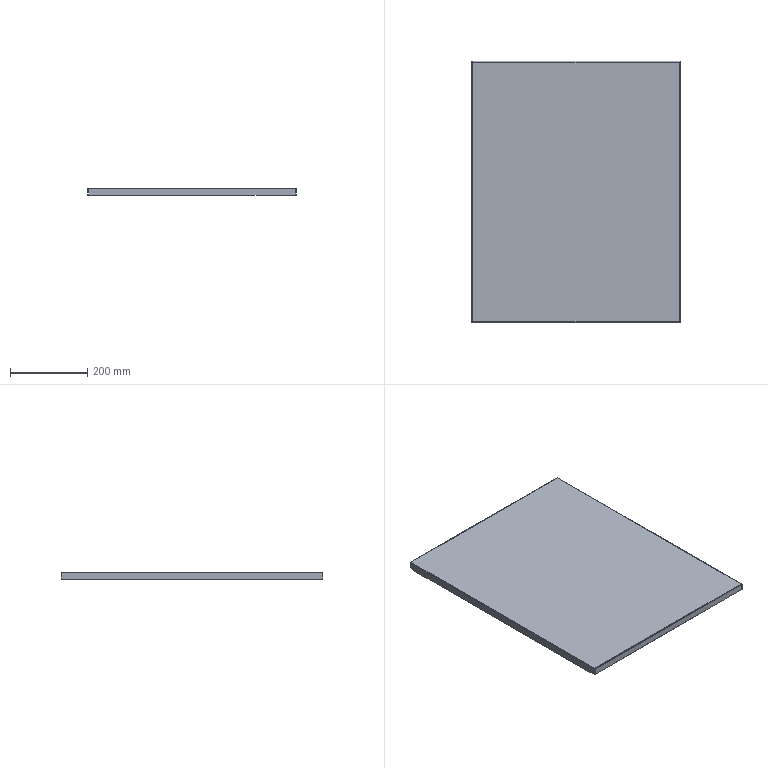Part | SolidWorks | features BaseBody 1 | 1 solid | 50 faces | box 537.5 x 674.5 x 20 mm | volume 485472 mm3 | plane 42 | cylinder 8 | commonest cylinder face diameters 1 x4 3.4 x4
STEP:
#1=CARTESIAN_POINT('',(-267.55,-319.25,-20.));
#2=VERTEX_POINT('',#1);
#3=CARTESIAN_POINT('',(-268.75,-319.25,-20.));
#4=VERTEX_POINT('',#3);
#5=CARTESIAN_POINT('',(268.75,-319.25,-20.));
#6=DIRECTION('',(-1.,0.,0.));
#7=VECTOR('',#6,1000.);
#8=LINE('',#5,#7);
#9=EDGE_CURVE('',#2,#4,#8,.T.);
#10=ORIENTED_EDGE('',*,*,#9,.F.);
#11=CARTESIAN_POINT('',(-267.55,-319.25,-18.));
#12=VERTEX_POINT('',#11);
#13=CARTESIAN_POINT('',(-267.55,-319.25,0.));
#14=DIRECTION('',(0.,0.,1.));
#15=VECTOR('',#14,1000.);
#16=LINE('',#13,#15);
#17=EDGE_CURVE('',#2,#12,#16,.T.);
#18=ORIENTED_EDGE('',*,*,#17,.T.);
#19=CARTESIAN_POINT('',(-268.75,-319.25,-18.));
#20=VERTEX_POINT('',#19);
#21=CARTESIAN_POINT('',(268.75,-319.25,-18.));
#22=DIRECTION('',(-1.,0.,0.));
#23=VECTOR('',#22,1000.);
#24=LINE('',#21,#23);
#25=EDGE_CURVE('',#12,#20,#24,.T.);
#26=ORIENTED_EDGE('',*,*,#25,.T.);
#27=CARTESIAN_POINT('',(-268.75,-319.25,0.));
#28=DIRECTION('',(0.,0.,1.));
#29=VECTOR('',#28,1000.);
#30=LINE('',#27,#29);
#31=EDGE_CURVE('',#4,#20,#30,.T.);
#32=ORIENTED_EDGE('',*,*,#31,.F.);
#33=EDGE_LOOP('',(#10,#18,#26,#32));
#34=FACE_OUTER_BOUND('',#33,.T.);
#35=CARTESIAN_POINT('',(268.75,-319.25,-20.));
#36=DIRECTION('',(0.,1.,0.));
#37=DIRECTION('',(1.,0.,0.));
#38=AXIS2_PLACEMENT_3D('',#35,#36,#37);
#39=PLANE('',#38);
#40=ADVANCED_FACE('',(#34),#39,.F.);
#41=ORIENTED_EDGE('',*,*,#25,.F.);
#42=CARTESIAN_POINT('',(-267.55,-337.25,-18.));
#43=VERTEX_POINT('',#42);
#44=CARTESIAN_POINT('',(-267.55,0.,-18.));
#45=DIRECTION('',(0.,-1.,0.));
#46=VECTOR('',#45,1000.);
#47=LINE('',#44,#46);
#48=EDGE_CURVE('',#12,#43,#47,.T.);
#49=ORIENTED_EDGE('',*,*,#48,.T.);
#50=CARTESIAN_POINT('',(-268.75,-337.25,-18.));
#51=VERTEX_POINT('',#50);
#52=CARTESIAN_POINT('',(268.75,-337.25,-18.));
#53=DIRECTION('',(-1.,0.,0.));
#54=VECTOR('',#53,1000.);
#55=LINE('',#52,#54);
#56=EDGE_CURVE('',#43,#51,#55,.T.);
#57=ORIENTED_EDGE('',*,*,#56,.T.);
#58=CARTESIAN_POINT('',(-268.75,0.,-18.));
#59=DIRECTION('',(0.,-1.,0.));
#60=VECTOR('',#59,1000.);
#61=LINE('',#58,#60);
#62=EDGE_CURVE('',#20,#51,#61,.T.);
#63=ORIENTED_EDGE('',*,*,#62,.F.);
#64=EDGE_LOOP('',(#41,#49,#57,#63));
#65=FACE_OUTER_BOUND('',#64,.T.);
#66=CARTESIAN_POINT('',(268.75,-337.25,-18.));
#67=DIRECTION('',(0.,0.,1.));
#68=DIRECTION('',(1.,0.,0.));
#69=AXIS2_PLACEMENT_3D('',#66,#67,#68);
#70=PLANE('',#69);
#71=ADVANCED_FACE('',(#65),#70,.F.);
#72=CARTESIAN_POINT('',(-267.55,319.25,-18.));
#73=VERTEX_POINT('',#72);
#74=CARTESIAN_POINT('',(-268.75,319.25,-18.));
#75=VERTEX_POINT('',#74);
#76=CARTESIAN_POINT('',(268.75,319.25,-18.));
#77=DIRECTION('',(-1.,0.,0.));
#78=VECTOR('',#77,1000.);
#79=LINE('',#76,#78);
#80=EDGE_CURVE('',#73,#75,#79,.T.);
#81=ORIENTED_EDGE('',*,*,#80,.F.);
#82=CARTESIAN_POINT('',(-267.55,319.25,-20.));
#83=VERTEX_POINT('',#82);
#84=CARTESIAN_POINT('',(-267.55,319.25,0.));
#85=DIRECTION('',(0.,0.,-1.));
#86=VECTOR('',#85,1000.);
#87=LINE('',#84,#86);
#88=EDGE_CURVE('',#73,#83,#87,.T.);
#89=ORIENTED_EDGE('',*,*,#88,.T.);
#90=CARTESIAN_POINT('',(-268.75,319.25,-20.));
#91=VERTEX_POINT('',#90);
#92=CARTESIAN_POINT('',(268.75,319.25,-20.));
#93=DIRECTION('',(-1.,0.,0.));
#94=VECTOR('',#93,1000.);
#95=LINE('',#92,#94);
#96=EDGE_CURVE('',#83,#91,#95,.T.);
#97=ORIENTED_EDGE('',*,*,#96,.T.);
#98=CARTESIAN_POINT('',(-268.75,319.25,0.));
#99=DIRECTION('',(0.,0.,-1.));
#100=VECTOR('',#99,1000.);
#101=LINE('',#98,#100);
#102=EDGE_CURVE('',#75,#91,#101,.T.);
#103=ORIENTED_EDGE('',*,*,#102,.F.);
#104=EDGE_LOOP('',(#81,#89,#97,#103));
#105=FACE_OUTER_BOUND('',#104,.T.);
#106=CARTESIAN_POINT('',(268.75,319.25,-20.));
#107=DIRECTION('',(0.,-1.,0.));
#108=DIRECTION('',(0.,0.,-1.));
#109=AXIS2_PLACEMENT_3D('',#106,#107,#108);
#110=PLANE('',#109);
#111=ADVANCED_FACE('',(#105),#110,.F.);
#112=CARTESIAN_POINT('',(-267.55,337.25,-18.));
#113=VERTEX_POINT('',#112);
#114=CARTESIAN_POINT('',(-268.75,337.25,-18.));
#115=VERTEX_POINT('',#114);
#116=CARTESIAN_POINT('',(268.75,337.25,-18.));
#117=DIRECTION('',(-1.,0.,0.));
#118=VECTOR('',#117,1000.);
#119=LINE('',#116,#118);
#120=EDGE_CURVE('',#113,#115,#119,.T.);
#121=ORIENTED_EDGE('',*,*,#120,.F.);
#122=CARTESIAN_POINT('',(-267.55,0.,-18.));
#123=DIRECTION('',(0.,-1.,0.));
#124=VECTOR('',#123,1000.);
#125=LINE('',#122,#124);
#126=EDGE_CURVE('',#113,#73,#125,.T.);
#127=ORIENTED_EDGE('',*,*,#126,.T.);
#128=ORIENTED_EDGE('',*,*,#80,.T.);
#129=CARTESIAN_POINT('',(-268.75,0.,-18.));
#130=DIRECTION('',(0.,-1.,0.));
#131=VECTOR('',#130,1000.);
#132=LINE('',#129,#131);
#133=EDGE_CURVE('',#115,#75,#132,.T.);
#134=ORIENTED_EDGE('',*,*,#133,.F.);
#135=EDGE_LOOP('',(#121,#127,#128,#134));
#136=FACE_OUTER_BOUND('',#135,.T.);
#137=CARTESIAN_POINT('',(268.75,337.25,-18.));
#138=DIRECTION('',(0.,0.,1.));
#139=DIRECTION('',(1.,0.,0.));
#140=AXIS2_PLACEMENT_3D('',#137,#138,#139);
#141=PLANE('',#140);
#142=ADVANCED_FACE('',(#136),#141,.F.);
#143=CARTESIAN_POINT('',(267.55,-335.55,-18.));
#144=VERTEX_POINT('',#143);
#145=CARTESIAN_POINT('',(267.55,-319.25,-18.));
#146=VERTEX_POINT('',#145);
#147=CARTESIAN_POINT('',(267.55,0.,-18.));
#148=DIRECTION('',(0.,1.,0.));
#149=VECTOR('',#148,1000.);
#150=LINE('',#147,#149);
#151=EDGE_CURVE('',#144,#146,#150,.T.);
#152=ORIENTED_EDGE('',*,*,#151,.T.);
#153=CARTESIAN_POINT('',(268.75,-319.25,-18.));
#154=VERTEX_POINT('',#153);
#155=CARTESIAN_POINT('',(268.75,-319.25,-18.));
#156=DIRECTION('',(-1.,0.,0.));
#157=VECTOR('',#156,1000.);
#158=LINE('',#155,#157);
#159=EDGE_CURVE('',#154,#146,#158,.T.);
#160=ORIENTED_EDGE('',*,*,#159,.F.);
#161=CARTESIAN_POINT('',(268.75,-335.55,-18.));
#162=VERTEX_POINT('',#161);
#163=CARTESIAN_POINT('',(268.75,-337.25,-18.));
#164=DIRECTION('',(0.,1.,0.));
#165=VECTOR('',#164,1000.);
#166=LINE('',#163,#165);
#167=EDGE_CURVE('',#162,#154,#166,.T.);
#168=ORIENTED_EDGE('',*,*,#167,.F.);
#169=CARTESIAN_POINT('',(268.75,-335.55,-18.));
#170=DIRECTION('',(1.,0.,0.));
#171=VECTOR('',#170,1000.);
#172=LINE('',#169,#171);
#173=EDGE_CURVE('',#144,#162,#172,.T.);
#174=ORIENTED_EDGE('',*,*,#173,.F.);
#175=EDGE_LOOP('',(#152,#160,#168,#174));
#176=FACE_OUTER_BOUND('',#175,.T.);
#177=CARTESIAN_POINT('',(268.75,-337.25,-18.));
#178=DIRECTION('',(0.,0.,1.));
#179=DIRECTION('',(1.,0.,0.));
#180=AXIS2_PLACEMENT_3D('',#177,#178,#179);
#181=PLANE('',#180);
#182=ADVANCED_FACE('',(#176),#181,.F.);
#183=CARTESIAN_POINT('',(267.55,-319.25,-20.));
#184=VERTEX_POINT('',#183);
#185=CARTESIAN_POINT('',(267.55,-319.25,0.));
#186=DIRECTION('',(0.,0.,-1.));
#187=VECTOR('',#186,1000.);
#188=LINE('',#185,#187);
#189=EDGE_CURVE('',#146,#184,#188,.T.);
#190=ORIENTED_EDGE('',*,*,#189,.T.);
#191=CARTESIAN_POINT('',(268.75,-319.25,-20.));
#192=VERTEX_POINT('',#191);
#193=CARTESIAN_POINT('',(268.75,-319.25,-20.));
#194=DIRECTION('',(-1.,0.,0.));
#195=VECTOR('',#194,1000.);
#196=LINE('',#193,#195);
#197=EDGE_CURVE('',#192,#184,#196,.T.);
#198=ORIENTED_EDGE('',*,*,#197,.F.);
#199=CARTESIAN_POINT('',(268.75,-319.25,-20.));
#200=DIRECTION('',(0.,0.,-1.));
#201=VECTOR('',#200,1000.);
#202=LINE('',#199,#201);
#203=EDGE_CURVE('',#154,#192,#202,.T.);
#204=ORIENTED_EDGE('',*,*,#203,.F.);
#205=ORIENTED_EDGE('',*,*,#159,.T.);
#206=EDGE_LOOP('',(#190,#198,#204,#205));
#207=FACE_OUTER_BOUND('',#206,.T.);
#208=CARTESIAN_POINT('',(268.75,-319.25,-20.));
#209=DIRECTION('',(0.,1.,0.));
#210=DIRECTION('',(1.,0.,0.));
#211=AXIS2_PLACEMENT_3D('',#208,#209,#210);
#212=PLANE('',#211);
#213=ADVANCED_FACE('',(#207),#212,.F.);
#214=CARTESIAN_POINT('',(268.75,319.25,-18.));
#215=VERTEX_POINT('',#214);
#216=CARTESIAN_POINT('',(268.75,335.55,-18.));
#217=VERTEX_POINT('',#216);
#218=CARTESIAN_POINT('',(268.75,337.25,-18.));
#219=DIRECTION('',(0.,1.,0.));
#220=VECTOR('',#219,1000.);
#221=LINE('',#218,#220);
#222=EDGE_CURVE('',#215,#217,#221,.T.);
#223=ORIENTED_EDGE('',*,*,#222,.F.);
#224=CARTESIAN_POINT('',(267.55,319.25,-18.));
#225=VERTEX_POINT('',#224);
#226=CARTESIAN_POINT('',(268.75,319.25,-18.));
#227=DIRECTION('',(-1.,0.,0.));
#228=VECTOR('',#227,1000.);
#229=LINE('',#226,#228);
#230=EDGE_CURVE('',#215,#225,#229,.T.);
#231=ORIENTED_EDGE('',*,*,#230,.T.);
#232=CARTESIAN_POINT('',(267.55,335.55,-18.));
#233=VERTEX_POINT('',#232);
#234=CARTESIAN_POINT('',(267.55,0.,-18.));
#235=DIRECTION('',(0.,1.,0.));
#236=VECTOR('',#235,1000.);
#237=LINE('',#234,#236);
#238=EDGE_CURVE('',#225,#233,#237,.T.);
#239=ORIENTED_EDGE('',*,*,#238,.T.);
#240=CARTESIAN_POINT('',(268.75,335.55,-18.));
#241=DIRECTION('',(-1.,0.,0.));
#242=VECTOR('',#241,1000.);
#243=LINE('',#240,#242);
#244=EDGE_CURVE('',#217,#233,#243,.T.);
#245=ORIENTED_EDGE('',*,*,#244,.F.);
#246=EDGE_LOOP('',(#223,#231,#239,#245));
#247=FACE_OUTER_BOUND('',#246,.T.);
#248=CARTESIAN_POINT('',(268.75,337.25,-18.));
#249=DIRECTION('',(0.,0.,1.));
#250=DIRECTION('',(1.,0.,0.));
#251=AXIS2_PLACEMENT_3D('',#248,#249,#250);
#252=PLANE('',#251);
#253=ADVANCED_FACE('',(#247),#252,.F.);
#254=CARTESIAN_POINT('',(267.55,319.25,-20.));
#255=VERTEX_POINT('',#254);
#256=CARTESIAN_POINT('',(267.55,319.25,0.));
#257=DIRECTION('',(0.,0.,1.));
#258=VECTOR('',#257,1000.);
#259=LINE('',#256,#258);
#260=EDGE_CURVE('',#255,#225,#259,.T.);
#261=ORIENTED_EDGE('',*,*,#260,.T.);
#262=ORIENTED_EDGE('',*,*,#230,.F.);
#263=CARTESIAN_POINT('',(268.75,319.25,-20.));
#264=VERTEX_POINT('',#263);
#265=CARTESIAN_POINT('',(268.75,319.25,-20.));
#266=DIRECTION('',(0.,0.,1.));
#267=VECTOR('',#266,1000.);
#268=LINE('',#265,#267);
#269=EDGE_CURVE('',#264,#215,#268,.T.);
#270=ORIENTED_EDGE('',*,*,#269,.F.);
#271=CARTESIAN_POINT('',(268.75,319.25,-20.));
#272=DIRECTION('',(-1.,0.,0.));
#273=VECTOR('',#272,1000.);
#274=LINE('',#271,#273);
#275=EDGE_CURVE('',#264,#255,#274,.T.);
#276=ORIENTED_EDGE('',*,*,#275,.T.);
#277=EDGE_LOOP('',(#261,#262,#270,#276));
#278=FACE_OUTER_BOUND('',#277,.T.);
#279=CARTESIAN_POINT('',(268.75,319.25,-20.));
#280=DIRECTION('',(0.,-1.,0.));
#281=DIRECTION('',(0.,0.,-1.));
#282=AXIS2_PLACEMENT_3D('',#279,#280,#281);
#283=PLANE('',#282);
#284=ADVANCED_FACE('',(#278),#283,.F.);
#285=CARTESIAN_POINT('',(268.75,0.,-20.));
#286=DIRECTION('',(0.,1.,0.));
#287=VECTOR('',#286,1000.);
#288=LINE('',#285,#287);
#289=EDGE_CURVE('',#192,#264,#288,.T.);
#290=ORIENTED_EDGE('',*,*,#289,.F.);
#291=ORIENTED_EDGE('',*,*,#197,.T.);
#292=CARTESIAN_POINT('',(267.55,335.55,-20.));
#293=DIRECTION('',(0.,1.,0.));
#294=VECTOR('',#293,1000.);
#295=LINE('',#292,#294);
#296=EDGE_CURVE('',#184,#255,#295,.T.);
#297=ORIENTED_EDGE('',*,*,#296,.T.);
#298=ORIENTED_EDGE('',*,*,#275,.F.);
#299=EDGE_LOOP('',(#290,#291,#297,#298));
#300=FACE_OUTER_BOUND('',#299,.T.);
#301=CARTESIAN_POINT('',(268.75,335.55,-20.));
#302=DIRECTION('',(0.,0.,1.));
#303=DIRECTION('',(1.,0.,0.));
#304=AXIS2_PLACEMENT_3D('',#301,#302,#303);
#305=PLANE('',#304);
#306=ADVANCED_FACE('',(#300),#305,.F.);
#307=ORIENTED_EDGE('',*,*,#189,.F.);
#308=ORIENTED_EDGE('',*,*,#151,.F.);
#309=CARTESIAN_POINT('',(267.55,-335.55,-1.7));
#310=VERTEX_POINT('',#309);
#311=CARTESIAN_POINT('',(267.55,-335.55,-20.));
#312=DIRECTION('',(0.,0.,-1.));
#313=VECTOR('',#312,1000.);
#314=LINE('',#311,#313);
#315=EDGE_CURVE('',#310,#144,#314,.T.);
#316=ORIENTED_EDGE('',*,*,#315,.F.);
#317=CARTESIAN_POINT('',(267.55,335.55,-1.7));
#318=VERTEX_POINT('',#317);
#319=CARTESIAN_POINT('',(267.55,335.55,-1.7));
#320=DIRECTION('',(0.,-1.,0.));
#321=VECTOR('',#320,1000.);
#322=LINE('',#319,#321);
#323=EDGE_CURVE('',#318,#310,#322,.T.);
#324=ORIENTED_EDGE('',*,*,#323,.F.);
#325=CARTESIAN_POINT('',(267.55,335.55,-1.2));
#326=DIRECTION('',(0.,0.,1.));
#327=VECTOR('',#326,1000.);
#328=LINE('',#325,#327);
#329=EDGE_CURVE('',#233,#318,#328,.T.);
#330=ORIENTED_EDGE('',*,*,#329,.F.);
#331=ORIENTED_EDGE('',*,*,#238,.F.);
#332=ORIENTED_EDGE('',*,*,#260,.F.);
#333=ORIENTED_EDGE('',*,*,#296,.F.);
#334=EDGE_LOOP('',(#307,#308,#316,#324,#330,#331,#332,#333));
#335=FACE_OUTER_BOUND('',#334,.T.);
#336=CARTESIAN_POINT('',(267.55,0.,0.));
#337=DIRECTION('',(-1.,0.,0.));
#338=DIRECTION('',(0.,0.,1.));
#339=AXIS2_PLACEMENT_3D('',#336,#337,#338);
#340=PLANE('',#339);
#341=ADVANCED_FACE('',(#335),#340,.T.);
#342=ORIENTED_EDGE('',*,*,#167,.T.);
#343=ORIENTED_EDGE('',*,*,#203,.T.);
#344=ORIENTED_EDGE('',*,*,#289,.T.);
#345=ORIENTED_EDGE('',*,*,#269,.T.);
#346=ORIENTED_EDGE('',*,*,#222,.T.);
#347=CARTESIAN_POINT('',(268.75,335.55,-1.7));
#348=VERTEX_POINT('',#347);
#349=CARTESIAN_POINT('',(268.75,335.55,0.));
#350=DIRECTION('',(0.,0.,1.));
#351=VECTOR('',#350,1000.);
#352=LINE('',#349,#351);
#353=EDGE_CURVE('',#217,#348,#352,.T.);
#354=ORIENTED_EDGE('',*,*,#353,.T.);
#355=CARTESIAN_POINT('',(268.75,-335.55,-1.7));
#356=VERTEX_POINT('',#355);
#357=CARTESIAN_POINT('',(268.75,335.55,-1.7));
#358=DIRECTION('',(0.,1.,0.));
#359=VECTOR('',#358,1000.);
#360=LINE('',#357,#359);
#361=EDGE_CURVE('',#356,#348,#360,.T.);
#362=ORIENTED_EDGE('',*,*,#361,.F.);
#363=CARTESIAN_POINT('',(268.75,-335.55,0.));
#364=DIRECTION('',(0.,0.,-1.));
#365=VECTOR('',#364,1000.);
#366=LINE('',#363,#365);
#367=EDGE_CURVE('',#356,#162,#366,.T.);
#368=ORIENTED_EDGE('',*,*,#367,.T.);
#369=EDGE_LOOP('',(#342,#343,#344,#345,#346,#354,#362,#368));
#370=FACE_OUTER_BOUND('',#369,.T.);
#371=CARTESIAN_POINT('',(268.75,0.,0.));
#372=DIRECTION('',(-1.,0.,0.));
#373=DIRECTION('',(0.,0.,1.));
#374=AXIS2_PLACEMENT_3D('',#371,#372,#373);
#375=PLANE('',#374);
#376=ADVANCED_FACE('',(#370),#375,.F.);
#377=ORIENTED_EDGE('',*,*,#353,.F.);
#378=ORIENTED_EDGE('',*,*,#244,.T.);
#379=ORIENTED_EDGE('',*,*,#329,.T.);
#380=CARTESIAN_POINT('',(268.75,335.55,-1.7));
#381=DIRECTION('',(1.,0.,0.));
#382=VECTOR('',#381,1000.);
#383=LINE('',#380,#382);
#384=EDGE_CURVE('',#318,#348,#383,.T.);
#385=ORIENTED_EDGE('',*,*,#384,.T.);
#386=EDGE_LOOP('',(#377,#378,#379,#385));
#387=FACE_OUTER_BOUND('',#386,.T.);
#388=CARTESIAN_POINT('',(268.75,335.55,-1.2));
#389=DIRECTION('',(0.,-1.,0.));
#390=DIRECTION('',(0.,0.,-1.));
#391=AXIS2_PLACEMENT_3D('',#388,#389,#390);
#392=PLANE('',#391);
#393=ADVANCED_FACE('',(#387),#392,.F.);
#394=ORIENTED_EDGE('',*,*,#315,.T.);
#395=ORIENTED_EDGE('',*,*,#173,.T.);
#396=ORIENTED_EDGE('',*,*,#367,.F.);
#397=CARTESIAN_POINT('',(267.55,-335.55,-1.7));
#398=DIRECTION('',(1.,0.,0.));
#399=VECTOR('',#398,1000.);
#400=LINE('',#397,#399);
#401=EDGE_CURVE('',#310,#356,#400,.T.);
#402=ORIENTED_EDGE('',*,*,#401,.F.);
#403=EDGE_LOOP('',(#394,#395,#396,#402));
#404=FACE_OUTER_BOUND('',#403,.T.);
#405=CARTESIAN_POINT('',(268.75,-335.55,-20.));
#406=DIRECTION('',(0.,1.,0.));
#407=DIRECTION('',(1.,0.,0.));
#408=AXIS2_PLACEMENT_3D('',#405,#406,#407);
#409=PLANE('',#408);
#410=ADVANCED_FACE('',(#404),#409,.F.);
#411=CARTESIAN_POINT('',(267.05,-335.55,-1.2));
#412=VERTEX_POINT('',#411);
#413=CARTESIAN_POINT('',(267.05,335.55,-1.2));
#414=VERTEX_POINT('',#413);
#415=CARTESIAN_POINT('',(267.05,-335.55,-1.2));
#416=DIRECTION('',(0.,1.,0.));
#417=VECTOR('',#416,1000.);
#418=LINE('',#415,#417);
#419=EDGE_CURVE('',#412,#414,#418,.T.);
#420=ORIENTED_EDGE('',*,*,#419,.T.);
#421=CARTESIAN_POINT('',(267.05,335.55,-1.7));
#422=DIRECTION('',(0.,1.,0.));
#423=DIRECTION('',(0.,0.,-1.));
#424=AXIS2_PLACEMENT_3D('',#421,#422,#423);
#425=CIRCLE('',#424,0.5);
#426=EDGE_CURVE('',#414,#318,#425,.T.);
#427=ORIENTED_EDGE('',*,*,#426,.T.);
#428=ORIENTED_EDGE('',*,*,#323,.T.);
#429=CARTESIAN_POINT('',(267.05,-335.55,-1.7));
#430=DIRECTION('',(0.,-1.,0.));
#431=DIRECTION('',(0.,0.,-1.));
#432=AXIS2_PLACEMENT_3D('',#429,#430,#431);
#433=CIRCLE('',#432,0.5);
#434=EDGE_CURVE('',#310,#412,#433,.T.);
#435=ORIENTED_EDGE('',*,*,#434,.T.);
#436=EDGE_LOOP('',(#420,#427,#428,#435));
#437=FACE_OUTER_BOUND('',#436,.T.);
#438=CARTESIAN_POINT('',(267.05,-335.55,-1.7));
#439=DIRECTION('',(0.,-1.,0.));
#440=DIRECTION('',(1.,0.,0.));
#441=AXIS2_PLACEMENT_3D('',#438,#439,#440);
#442=CYLINDRICAL_SURFACE('',#441,0.5);
#443=ADVANCED_FACE('',(#437),#442,.F.);
#444=CARTESIAN_POINT('',(267.05,-335.55,0.));
#445=VERTEX_POINT('',#444);
#446=CARTESIAN_POINT('',(267.05,335.55,0.));
#447=VERTEX_POINT('',#446);
#448=CARTESIAN_POINT('',(267.05,-335.55,0.));
#449=DIRECTION('',(0.,1.,0.));
#450=VECTOR('',#449,1000.);
#451=LINE('',#448,#450);
#452=EDGE_CURVE('',#445,#447,#451,.T.);
#453=ORIENTED_EDGE('',*,*,#452,.F.);
#454=CARTESIAN_POINT('',(268.675,-335.55,-1.2));
#455=VERTEX_POINT('',#454);
#456=CARTESIAN_POINT('',(267.05,-335.55,-1.7));
#457=DIRECTION('',(0.,-1.,0.));
#458=DIRECTION('',(0.,0.,-1.));
#459=AXIS2_PLACEMENT_3D('',#456,#457,#458);
#460=CIRCLE('',#459,1.7);
#461=EDGE_CURVE('',#455,#445,#460,.T.);
#462=ORIENTED_EDGE('',*,*,#461,.F.);
#463=CARTESIAN_POINT('',(267.05,-335.55,-1.7));
#464=DIRECTION('',(0.,-1.,0.));
#465=DIRECTION('',(0.,0.,-1.));
#466=AXIS2_PLACEMENT_3D('',#463,#464,#465);
#467=CIRCLE('',#466,1.7);
#468=EDGE_CURVE('',#356,#455,#467,.T.);
#469=ORIENTED_EDGE('',*,*,#468,.F.);
#470=ORIENTED_EDGE('',*,*,#361,.T.);
#471=CARTESIAN_POINT('',(268.675,335.55,-1.2));
#472=VERTEX_POINT('',#471);
#473=CARTESIAN_POINT('',(267.05,335.55,-1.7));
#474=DIRECTION('',(0.,1.,0.));
#475=DIRECTION('',(0.,0.,-1.));
#476=AXIS2_PLACEMENT_3D('',#473,#474,#475);
#477=CIRCLE('',#476,1.7);
#478=EDGE_CURVE('',#472,#348,#477,.T.);
#479=ORIENTED_EDGE('',*,*,#478,.F.);
#480=CARTESIAN_POINT('',(267.05,335.55,-1.7));
#481=DIRECTION('',(0.,1.,0.));
#482=DIRECTION('',(0.,0.,-1.));
#483=AXIS2_PLACEMENT_3D('',#480,#481,#482);
#484=CIRCLE('',#483,1.7);
#485=EDGE_CURVE('',#447,#472,#484,.T.);
#486=ORIENTED_EDGE('',*,*,#485,.F.);
#487=EDGE_LOOP('',(#453,#462,#469,#470,#479,#486));
#488=FACE_OUTER_BOUND('',#487,.T.);
#489=CARTESIAN_POINT('',(267.05,-335.55,-1.7));
#490=DIRECTION('',(0.,-1.,0.));
#491=DIRECTION('',(1.,0.,0.));
#492=AXIS2_PLACEMENT_3D('',#489,#490,#491);
#493=CYLINDRICAL_SURFACE('',#492,1.7);
#494=ADVANCED_FACE('',(#488),#493,.T.);
#495=ORIENTED_EDGE('',*,*,#468,.T.);
#496=CARTESIAN_POINT('',(268.75,-335.55,-1.2));
#497=DIRECTION('',(-1.,0.,0.));
#498=VECTOR('',#497,1000.);
#499=LINE('',#496,#498);
#500=EDGE_CURVE('',#455,#412,#499,.T.);
#501=ORIENTED_EDGE('',*,*,#500,.T.);
#502=ORIENTED_EDGE('',*,*,#434,.F.);
#503=ORIENTED_EDGE('',*,*,#401,.T.);
#504=EDGE_LOOP('',(#495,#501,#502,#503));
#505=FACE_OUTER_BOUND('',#504,.T.);
#506=CARTESIAN_POINT('',(267.05,-335.55,-1.7));
#507=DIRECTION('',(0.,1.,0.));
#508=DIRECTION('',(0.,0.,-1.));
#509=AXIS2_PLACEMENT_3D('',#506,#507,#508);
#510=PLANE('',#509);
#511=ADVANCED_FACE('',(#505),#510,.F.);
#512=CARTESIAN_POINT('',(268.75,335.55,-1.2));
#513=DIRECTION('',(-1.,0.,0.));
#514=VECTOR('',#513,1000.);
#515=LINE('',#512,#514);
#516=EDGE_CURVE('',#472,#414,#515,.T.);
#517=ORIENTED_EDGE('',*,*,#516,.F.);
#518=ORIENTED_EDGE('',*,*,#478,.T.);
#519=ORIENTED_EDGE('',*,*,#384,.F.);
#520=ORIENTED_EDGE('',*,*,#426,.F.);
#521=EDGE_LOOP('',(#517,#518,#519,#520));
#522=FACE_OUTER_BOUND('',#521,.T.);
#523=CARTESIAN_POINT('',(267.05,335.55,-1.7));
#524=DIRECTION('',(0.,1.,0.));
#525=DIRECTION('',(0.,0.,-1.));
#526=AXIS2_PLACEMENT_3D('',#523,#524,#525);
#527=PLANE('',#526);
#528=ADVANCED_FACE('',(#522),#527,.T.);
#529=CARTESIAN_POINT('',(268.75,336.05,-18.));
#530=VERTEX_POINT('',#529);
#531=CARTESIAN_POINT('',(-267.05,336.05,-18.));
#532=VERTEX_POINT('',#531);
#533=CARTESIAN_POINT('',(-267.05,336.05,-18.));
#534=DIRECTION('',(-1.,0.,0.));
#535=VECTOR('',#534,1000.);
#536=LINE('',#533,#535);
#537=EDGE_CURVE('',#530,#532,#536,.T.);
#538=ORIENTED_EDGE('',*,*,#537,.T.);
#539=CARTESIAN_POINT('',(-267.05,337.25,-18.));
#540=VERTEX_POINT('',#539);
#541=CARTESIAN_POINT('',(-267.05,337.25,-18.));
#542=DIRECTION('',(0.,-1.,0.));
#543=VECTOR('',#542,1000.);
#544=LINE('',#541,#543);
#545=EDGE_CURVE('',#540,#532,#544,.T.);
#546=ORIENTED_EDGE('',*,*,#545,.F.);
#547=CARTESIAN_POINT('',(268.75,337.25,-18.));
#548=VERTEX_POINT('',#547);
#549=CARTESIAN_POINT('',(0.,337.25,-18.));
#550=DIRECTION('',(-1.,0.,0.));
#551=VECTOR('',#550,1000.);
#552=LINE('',#549,#551);
#553=EDGE_CURVE('',#548,#540,#552,.T.);
#554=ORIENTED_EDGE('',*,*,#553,.F.);
#555=CARTESIAN_POINT('',(268.75,337.25,-18.));
#556=DIRECTION('',(0.,-1.,0.));
#557=VECTOR('',#556,1000.);
#558=LINE('',#555,#557);
#559=EDGE_CURVE('',#548,#530,#558,.T.);
#560=ORIENTED_EDGE('',*,*,#559,.T.);
#561=EDGE_LOOP('',(#538,#546,#554,#560));
#562=FACE_OUTER_BOUND('',#561,.T.);
#563=CARTESIAN_POINT('',(-267.05,337.25,-18.));
#564=DIRECTION('',(0.,0.,1.));
#565=DIRECTION('',(0.,-1.,0.));
#566=AXIS2_PLACEMENT_3D('',#563,#564,#565);
#567=PLANE('',#566);
#568=ADVANCED_FACE('',(#562),#567,.F.);
#569=CARTESIAN_POINT('',(268.75,336.05,-1.7));
#570=VERTEX_POINT('',#569);
#571=CARTESIAN_POINT('',(268.75,336.05,-18.));
#572=DIRECTION('',(0.,0.,-1.));
#573=VECTOR('',#572,1000.);
#574=LINE('',#571,#573);
#575=EDGE_CURVE('',#570,#530,#574,.T.);
#576=ORIENTED_EDGE('',*,*,#575,.F.);
#577=CARTESIAN_POINT('',(-267.05,336.05,-1.7));
#578=VERTEX_POINT('',#577);
#579=CARTESIAN_POINT('',(-267.05,336.05,-1.7));
#580=DIRECTION('',(1.,0.,0.));
#581=VECTOR('',#580,1000.);
#582=LINE('',#579,#581);
#583=EDGE_CURVE('',#578,#570,#582,.T.);
#584=ORIENTED_EDGE('',*,*,#583,.F.);
#585=CARTESIAN_POINT('',(-267.05,336.05,-1.2));
#586=DIRECTION('',(0.,0.,1.));
#587=VECTOR('',#586,1000.);
#588=LINE('',#585,#587);
#589=EDGE_CURVE('',#532,#578,#588,.T.);
#590=ORIENTED_EDGE('',*,*,#589,.F.);
#591=ORIENTED_EDGE('',*,*,#537,.F.);
#592=EDGE_LOOP('',(#576,#584,#590,#591));
#593=FACE_OUTER_BOUND('',#592,.T.);
#594=CARTESIAN_POINT('',(0.,336.05,0.));
#595=DIRECTION('',(0.,-1.,0.));
#596=DIRECTION('',(0.,0.,-1.));
#597=AXIS2_PLACEMENT_3D('',#594,#595,#596);
#598=PLANE('',#597);
#599=ADVANCED_FACE('',(#593),#598,.T.);
#600=CARTESIAN_POINT('',(268.75,337.25,-1.7));
#601=VERTEX_POINT('',#600);
#602=CARTESIAN_POINT('',(-267.05,337.25,-1.7));
#603=VERTEX_POINT('',#602);
#604=CARTESIAN_POINT('',(-267.05,337.25,-1.7));
#605=DIRECTION('',(-1.,0.,0.));
#606=VECTOR('',#605,1000.);
#607=LINE('',#604,#606);
#608=EDGE_CURVE('',#601,#603,#607,.T.);
#609=ORIENTED_EDGE('',*,*,#608,.F.);
#610=CARTESIAN_POINT('',(268.75,337.25,0.));
#611=DIRECTION('',(0.,0.,-1.));
#612=VECTOR('',#611,1000.);
#613=LINE('',#610,#612);
#614=EDGE_CURVE('',#601,#548,#613,.T.);
#615=ORIENTED_EDGE('',*,*,#614,.T.);
#616=ORIENTED_EDGE('',*,*,#553,.T.);
#617=CARTESIAN_POINT('',(-267.05,337.25,0.));
#618=DIRECTION('',(0.,0.,1.));
#619=VECTOR('',#618,1000.);
#620=LINE('',#617,#619);
#621=EDGE_CURVE('',#540,#603,#620,.T.);
#622=ORIENTED_EDGE('',*,*,#621,.T.);
#623=EDGE_LOOP('',(#609,#615,#616,#622));
#624=FACE_OUTER_BOUND('',#623,.T.);
#625=CARTESIAN_POINT('',(0.,337.25,0.));
#626=DIRECTION('',(0.,-1.,0.));
#627=DIRECTION('',(0.,0.,-1.));
#628=AXIS2_PLACEMENT_3D('',#625,#626,#627);
#629=PLANE('',#628);
#630=ADVANCED_FACE('',(#624),#629,.F.);
#631=CARTESIAN_POINT('',(-267.05,337.25,-1.7));
#632=DIRECTION('',(0.,1.,0.));
#633=VECTOR('',#632,1000.);
#634=LINE('',#631,#633);
#635=EDGE_CURVE('',#578,#603,#634,.T.);
#636=ORIENTED_EDGE('',*,*,#635,.T.);
#637=ORIENTED_EDGE('',*,*,#621,.F.);
#638=ORIENTED_EDGE('',*,*,#545,.T.);
#639=ORIENTED_EDGE('',*,*,#589,.T.);
#640=EDGE_LOOP('',(#636,#637,#638,#639));
#641=FACE_OUTER_BOUND('',#640,.T.);
#642=CARTESIAN_POINT('',(-267.05,337.25,-1.2));
#643=DIRECTION('',(1.,0.,0.));
#644=DIRECTION('',(0.,1.,0.));
#645=AXIS2_PLACEMENT_3D('',#642,#643,#644);
#646=PLANE('',#645);
#647=ADVANCED_FACE('',(#641),#646,.F.);
#648=CARTESIAN_POINT('',(268.75,336.05,-1.7));
#649=DIRECTION('',(0.,1.,0.));
#650=VECTOR('',#649,1000.);
#651=LINE('',#648,#650);
#652=EDGE_CURVE('',#570,#601,#651,.T.);
#653=ORIENTED_EDGE('',*,*,#652,.F.);
#654=ORIENTED_EDGE('',*,*,#575,.T.);
#655=ORIENTED_EDGE('',*,*,#559,.F.);
#656=ORIENTED_EDGE('',*,*,#614,.F.);
#657=EDGE_LOOP('',(#653,#654,#655,#656));
#658=FACE_OUTER_BOUND('',#657,.T.);
#659=CARTESIAN_POINT('',(268.75,337.25,-18.));
#660=DIRECTION('',(-1.,0.,0.));
#661=DIRECTION('',(0.,1.,0.));
#662=AXIS2_PLACEMENT_3D('',#659,#660,#661);
#663=PLANE('',#662);
#664=ADVANCED_FACE('',(#658),#663,.F.);
#665=CARTESIAN_POINT('',(268.75,335.55,-1.2));
#666=VERTEX_POINT('',#665);
#667=CARTESIAN_POINT('',(268.75,335.55,-1.2));
#668=DIRECTION('',(-1.,0.,0.));
#669=VECTOR('',#668,1000.);
#670=LINE('',#667,#669);
#671=EDGE_CURVE('',#666,#472,#670,.T.);
#672=ORIENTED_EDGE('',*,*,#671,.T.);
#673=ORIENTED_EDGE('',*,*,#516,.T.);
#674=CARTESIAN_POINT('',(-267.05,335.55,-1.2));
#675=VERTEX_POINT('',#674);
#676=CARTESIAN_POINT('',(268.75,335.55,-1.2));
#677=DIRECTION('',(-1.,0.,0.));
#678=VECTOR('',#677,1000.);
#679=LINE('',#676,#678);
#680=EDGE_CURVE('',#414,#675,#679,.T.);
#681=ORIENTED_EDGE('',*,*,#680,.T.);
#682=CARTESIAN_POINT('',(-267.05,335.55,-1.7));
#683=DIRECTION('',(-1.,0.,0.));
#684=DIRECTION('',(0.,0.,-1.));
#685=AXIS2_PLACEMENT_3D('',#682,#683,#684);
#686=CIRCLE('',#685,0.5);
#687=EDGE_CURVE('',#675,#578,#686,.T.);
#688=ORIENTED_EDGE('',*,*,#687,.T.);
#689=ORIENTED_EDGE('',*,*,#583,.T.);
#690=CARTESIAN_POINT('',(268.75,335.55,-1.7));
#691=DIRECTION('',(1.,0.,0.));
#692=DIRECTION('',(0.,0.,-1.));
#693=AXIS2_PLACEMENT_3D('',#690,#691,#692);
#694=CIRCLE('',#693,0.5);
#695=EDGE_CURVE('',#570,#666,#694,.T.);
#696=ORIENTED_EDGE('',*,*,#695,.T.);
#697=EDGE_LOOP('',(#672,#673,#681,#688,#689,#696));
#698=FACE_OUTER_BOUND('',#697,.T.);
#699=CARTESIAN_POINT('',(268.75,335.55,-1.7));
#700=DIRECTION('',(1.,0.,0.));
#701=DIRECTION('',(0.,1.,0.));
#702=AXIS2_PLACEMENT_3D('',#699,#700,#701);
#703=CYLINDRICAL_SURFACE('',#702,0.5);
#704=ADVANCED_FACE('',(#698),#703,.F.);
#705=CARTESIAN_POINT('',(268.75,335.55,0.));
#706=VERTEX_POINT('',#705);
#707=CARTESIAN_POINT('',(268.75,335.55,0.));
#708=DIRECTION('',(-1.,0.,0.));
#709=VECTOR('',#708,1000.);
#710=LINE('',#707,#709);
#711=EDGE_CURVE('',#706,#447,#710,.T.);
#712=ORIENTED_EDGE('',*,*,#711,.F.);
#713=CARTESIAN_POINT('',(268.75,335.55,-1.7));
#714=DIRECTION('',(1.,0.,0.));
#715=DIRECTION('',(0.,0.,-1.));
#716=AXIS2_PLACEMENT_3D('',#713,#714,#715);
#717=CIRCLE('',#716,1.7);
#718=EDGE_CURVE('',#601,#706,#717,.T.);
#719=ORIENTED_EDGE('',*,*,#718,.F.);
#720=ORIENTED_EDGE('',*,*,#608,.T.);
#721=CARTESIAN_POINT('',(-267.05,335.55,0.));
#722=VERTEX_POINT('',#721);
#723=CARTESIAN_POINT('',(-267.05,335.55,-1.7));
#724=DIRECTION('',(-1.,0.,0.));
#725=DIRECTION('',(0.,0.,-1.));
#726=AXIS2_PLACEMENT_3D('',#723,#724,#725);
#727=CIRCLE('',#726,1.7);
#728=EDGE_CURVE('',#722,#603,#727,.T.);
#729=ORIENTED_EDGE('',*,*,#728,.F.);
#730=CARTESIAN_POINT('',(268.75,335.55,0.));
#731=DIRECTION('',(-1.,0.,0.));
#732=VECTOR('',#731,1000.);
#733=LINE('',#730,#732);
#734=EDGE_CURVE('',#447,#722,#733,.T.);
#735=ORIENTED_EDGE('',*,*,#734,.F.);
#736=EDGE_LOOP('',(#712,#719,#720,#729,#735));
#737=FACE_OUTER_BOUND('',#736,.T.);
#738=CARTESIAN_POINT('',(268.75,335.55,-1.7));
#739=DIRECTION('',(1.,0.,0.));
#740=DIRECTION('',(0.,1.,0.));
#741=AXIS2_PLACEMENT_3D('',#738,#739,#740);
#742=CYLINDRICAL_SURFACE('',#741,1.7);
#743=ADVANCED_FACE('',(#737),#742,.T.);
#744=ORIENTED_EDGE('',*,*,#695,.F.);
#745=ORIENTED_EDGE('',*,*,#652,.T.);
#746=ORIENTED_EDGE('',*,*,#718,.T.);
#747=CARTESIAN_POINT('',(268.75,335.55,-1.2));
#748=DIRECTION('',(0.,0.,1.));
#749=VECTOR('',#748,1000.);
#750=LINE('',#747,#749);
#751=EDGE_CURVE('',#666,#706,#750,.T.);
#752=ORIENTED_EDGE('',*,*,#751,.F.);
#753=EDGE_LOOP('',(#744,#745,#746,#752));
#754=FACE_OUTER_BOUND('',#753,.T.);
#755=CARTESIAN_POINT('',(268.75,335.55,-1.7));
#756=DIRECTION('',(-1.,0.,0.));
#757=DIRECTION('',(0.,0.,1.));
#758=AXIS2_PLACEMENT_3D('',#755,#756,#757);
#759=PLANE('',#758);
#760=ADVANCED_FACE('',(#754),#759,.F.);
#761=ORIENTED_EDGE('',*,*,#635,.F.);
#762=ORIENTED_EDGE('',*,*,#687,.F.);
#763=CARTESIAN_POINT('',(-267.05,335.55,-1.2));
#764=DIRECTION('',(0.,0.,1.));
#765=VECTOR('',#764,1000.);
#766=LINE('',#763,#765);
#767=EDGE_CURVE('',#675,#722,#766,.T.);
#768=ORIENTED_EDGE('',*,*,#767,.T.);
#769=ORIENTED_EDGE('',*,*,#728,.T.);
#770=EDGE_LOOP('',(#761,#762,#768,#769));
#771=FACE_OUTER_BOUND('',#770,.T.);
#772=CARTESIAN_POINT('',(-267.05,335.55,-1.7));
#773=DIRECTION('',(-1.,0.,0.));
#774=DIRECTION('',(0.,0.,1.));
#775=AXIS2_PLACEMENT_3D('',#772,#773,#774);
#776=PLANE('',#775);
#777=ADVANCED_FACE('',(#771),#776,.T.);
#778=CARTESIAN_POINT('',(-267.05,-336.05,-18.));
#779=VERTEX_POINT('',#778);
#780=CARTESIAN_POINT('',(268.75,-336.05,-18.));
#781=VERTEX_POINT('',#780);
#782=CARTESIAN_POINT('',(268.75,-336.05,-18.));
#783=DIRECTION('',(1.,0.,0.));
#784=VECTOR('',#783,1000.);
#785=LINE('',#782,#784);
#786=EDGE_CURVE('',#779,#781,#785,.T.);
#787=ORIENTED_EDGE('',*,*,#786,.T.);
#788=CARTESIAN_POINT('',(268.75,-337.25,-18.));
#789=VERTEX_POINT('',#788);
#790=CARTESIAN_POINT('',(268.75,-337.25,-18.));
#791=DIRECTION('',(0.,1.,0.));
#792=VECTOR('',#791,1000.);
#793=LINE('',#790,#792);
#794=EDGE_CURVE('',#789,#781,#793,.T.);
#795=ORIENTED_EDGE('',*,*,#794,.F.);
#796=CARTESIAN_POINT('',(-267.05,-337.25,-18.));
#797=VERTEX_POINT('',#796);
#798=CARTESIAN_POINT('',(0.,-337.25,-18.));
#799=DIRECTION('',(1.,0.,0.));
#800=VECTOR('',#799,1000.);
#801=LINE('',#798,#800);
#802=EDGE_CURVE('',#797,#789,#801,.T.);
#803=ORIENTED_EDGE('',*,*,#802,.F.);
#804=CARTESIAN_POINT('',(-267.05,-337.25,-18.));
#805=DIRECTION('',(0.,1.,0.));
#806=VECTOR('',#805,1000.);
#807=LINE('',#804,#806);
#808=EDGE_CURVE('',#797,#779,#807,.T.);
#809=ORIENTED_EDGE('',*,*,#808,.T.);
#810=EDGE_LOOP('',(#787,#795,#803,#809));
#811=FACE_OUTER_BOUND('',#810,.T.);
#812=CARTESIAN_POINT('',(268.75,-337.25,-18.));
#813=DIRECTION('',(0.,0.,1.));
#814=DIRECTION('',(0.,-1.,0.));
#815=AXIS2_PLACEMENT_3D('',#812,#813,#814);
#816=PLANE('',#815);
#817=ADVANCED_FACE('',(#811),#816,.F.);
#818=CARTESIAN_POINT('',(-267.05,-336.05,-1.7));
#819=VERTEX_POINT('',#818);
#820=CARTESIAN_POINT('',(-267.05,-336.05,-18.));
#821=DIRECTION('',(0.,0.,-1.));
#822=VECTOR('',#821,1000.);
#823=LINE('',#820,#822);
#824=EDGE_CURVE('',#819,#779,#823,.T.);
#825=ORIENTED_EDGE('',*,*,#824,.F.);
#826=CARTESIAN_POINT('',(268.75,-336.05,-1.7));
#827=VERTEX_POINT('',#826);
#828=CARTESIAN_POINT('',(268.75,-336.05,-1.7));
#829=DIRECTION('',(-1.,0.,0.));
#830=VECTOR('',#829,1000.);
#831=LINE('',#828,#830);
#832=EDGE_CURVE('',#827,#819,#831,.T.);
#833=ORIENTED_EDGE('',*,*,#832,.F.);
#834=CARTESIAN_POINT('',(268.75,-336.05,-1.2));
#835=DIRECTION('',(0.,0.,1.));
#836=VECTOR('',#835,1000.);
#837=LINE('',#834,#836);
#838=EDGE_CURVE('',#781,#827,#837,.T.);
#839=ORIENTED_EDGE('',*,*,#838,.F.);
#840=ORIENTED_EDGE('',*,*,#786,.F.);
#841=EDGE_LOOP('',(#825,#833,#839,#840));
#842=FACE_OUTER_BOUND('',#841,.T.);
#843=CARTESIAN_POINT('',(0.,-336.05,0.));
#844=DIRECTION('',(0.,1.,0.));
#845=DIRECTION('',(0.,0.,-1.));
#846=AXIS2_PLACEMENT_3D('',#843,#844,#845);
#847=PLANE('',#846);
#848=ADVANCED_FACE('',(#842),#847,.T.);
#849=CARTESIAN_POINT('',(-267.05,-337.25,-1.7));
#850=VERTEX_POINT('',#849);
#851=CARTESIAN_POINT('',(268.75,-337.25,-1.7));
#852=VERTEX_POINT('',#851);
#853=CARTESIAN_POINT('',(268.75,-337.25,-1.7));
#854=DIRECTION('',(1.,0.,0.));
#855=VECTOR('',#854,1000.);
#856=LINE('',#853,#855);
#857=EDGE_CURVE('',#850,#852,#856,.T.);
#858=ORIENTED_EDGE('',*,*,#857,.F.);
#859=CARTESIAN_POINT('',(-267.05,-337.25,0.));
#860=DIRECTION('',(0.,0.,-1.));
#861=VECTOR('',#860,1000.);
#862=LINE('',#859,#861);
#863=EDGE_CURVE('',#850,#797,#862,.T.);
#864=ORIENTED_EDGE('',*,*,#863,.T.);
#865=ORIENTED_EDGE('',*,*,#802,.T.);
#866=CARTESIAN_POINT('',(268.75,-337.25,0.));
#867=DIRECTION('',(0.,0.,1.));
#868=VECTOR('',#867,1000.);
#869=LINE('',#866,#868);
#870=EDGE_CURVE('',#789,#852,#869,.T.);
#871=ORIENTED_EDGE('',*,*,#870,.T.);
#872=EDGE_LOOP('',(#858,#864,#865,#871));
#873=FACE_OUTER_BOUND('',#872,.T.);
#874=CARTESIAN_POINT('',(0.,-337.25,0.));
#875=DIRECTION('',(0.,1.,0.));
#876=DIRECTION('',(0.,0.,-1.));
#877=AXIS2_PLACEMENT_3D('',#874,#875,#876);
#878=PLANE('',#877);
#879=ADVANCED_FACE('',(#873),#878,.F.);
#880=CARTESIAN_POINT('',(268.75,-337.25,-1.7));
#881=DIRECTION('',(0.,-1.,0.));
#882=VECTOR('',#881,1000.);
#883=LINE('',#880,#882);
#884=EDGE_CURVE('',#827,#852,#883,.T.);
#885=ORIENTED_EDGE('',*,*,#884,.T.);
#886=ORIENTED_EDGE('',*,*,#870,.F.);
#887=ORIENTED_EDGE('',*,*,#794,.T.);
#888=ORIENTED_EDGE('',*,*,#838,.T.);
#889=EDGE_LOOP('',(#885,#886,#887,#888));
#890=FACE_OUTER_BOUND('',#889,.T.);
#891=CARTESIAN_POINT('',(268.75,-337.25,-1.2));
#892=DIRECTION('',(-1.,0.,0.));
#893=DIRECTION('',(0.,0.,1.));
#894=AXIS2_PLACEMENT_3D('',#891,#892,#893);
#895=PLANE('',#894);
#896=ADVANCED_FACE('',(#890),#895,.F.);
#897=CARTESIAN_POINT('',(-267.05,-336.05,-1.7));
#898=DIRECTION('',(0.,-1.,0.));
#899=VECTOR('',#898,1000.);
#900=LINE('',#897,#899);
#901=EDGE_CURVE('',#819,#850,#900,.T.);
#902=ORIENTED_EDGE('',*,*,#901,.F.);
#903=ORIENTED_EDGE('',*,*,#824,.T.);
#904=ORIENTED_EDGE('',*,*,#808,.F.);
#905=ORIENTED_EDGE('',*,*,#863,.F.);
#906=EDGE_LOOP('',(#902,#903,#904,#905));
#907=FACE_OUTER_BOUND('',#906,.T.);
#908=CARTESIAN_POINT('',(-267.05,-337.25,-18.));
#909=DIRECTION('',(1.,0.,0.));
#910=DIRECTION('',(0.,1.,0.));
#911=AXIS2_PLACEMENT_3D('',#908,#909,#910);
#912=PLANE('',#911);
#913=ADVANCED_FACE('',(#907),#912,.F.);
#914=CARTESIAN_POINT('',(-267.05,-335.55,-1.2));
#915=VERTEX_POINT('',#914);
#916=CARTESIAN_POINT('',(-267.05,-335.55,-1.2));
#917=DIRECTION('',(1.,0.,0.));
#918=VECTOR('',#917,1000.);
#919=LINE('',#916,#918);
#920=EDGE_CURVE('',#915,#412,#919,.T.);
#921=ORIENTED_EDGE('',*,*,#920,.T.);
#922=ORIENTED_EDGE('',*,*,#500,.F.);
#923=CARTESIAN_POINT('',(268.75,-335.55,-1.2));
#924=VERTEX_POINT('',#923);
#925=CARTESIAN_POINT('',(268.75,-335.55,-1.2));
#926=DIRECTION('',(-1.,0.,0.));
#927=VECTOR('',#926,1000.);
#928=LINE('',#925,#927);
#929=EDGE_CURVE('',#924,#455,#928,.T.);
#930=ORIENTED_EDGE('',*,*,#929,.F.);
#931=CARTESIAN_POINT('',(268.75,-335.55,-1.7));
#932=DIRECTION('',(1.,0.,0.));
#933=DIRECTION('',(0.,0.,1.));
#934=AXIS2_PLACEMENT_3D('',#931,#932,#933);
#935=CIRCLE('',#934,0.5);
#936=EDGE_CURVE('',#924,#827,#935,.T.);
#937=ORIENTED_EDGE('',*,*,#936,.T.);
#938=ORIENTED_EDGE('',*,*,#832,.T.);
#939=CARTESIAN_POINT('',(-267.05,-335.55,-1.7));
#940=DIRECTION('',(-1.,0.,0.));
#941=DIRECTION('',(0.,0.,1.));
#942=AXIS2_PLACEMENT_3D('',#939,#940,#941);
#943=CIRCLE('',#942,0.5);
#944=EDGE_CURVE('',#819,#915,#943,.T.);
#945=ORIENTED_EDGE('',*,*,#944,.T.);
#946=EDGE_LOOP('',(#921,#922,#930,#937,#938,#945));
#947=FACE_OUTER_BOUND('',#946,.T.);
#948=CARTESIAN_POINT('',(-267.05,-335.55,-1.7));
#949=DIRECTION('',(-1.,0.,0.));
#950=DIRECTION('',(0.,-1.,0.));
#951=AXIS2_PLACEMENT_3D('',#948,#949,#950);
#952=CYLINDRICAL_SURFACE('',#951,0.5);
#953=ADVANCED_FACE('',(#947),#952,.F.);
#954=CARTESIAN_POINT('',(-267.05,-335.55,0.));
#955=VERTEX_POINT('',#954);
#956=CARTESIAN_POINT('',(-267.05,-335.55,0.));
#957=DIRECTION('',(1.,0.,0.));
#958=VECTOR('',#957,1000.);
#959=LINE('',#956,#958);
#960=EDGE_CURVE('',#955,#445,#959,.T.);
#961=ORIENTED_EDGE('',*,*,#960,.F.);
#962=CARTESIAN_POINT('',(-267.05,-335.55,-1.7));
#963=DIRECTION('',(-1.,0.,0.));
#964=DIRECTION('',(0.,0.,1.));
#965=AXIS2_PLACEMENT_3D('',#962,#963,#964);
#966=CIRCLE('',#965,1.7);
#967=EDGE_CURVE('',#850,#955,#966,.T.);
#968=ORIENTED_EDGE('',*,*,#967,.F.);
#969=ORIENTED_EDGE('',*,*,#857,.T.);
#970=CARTESIAN_POINT('',(268.75,-335.55,0.));
#971=VERTEX_POINT('',#970);
#972=CARTESIAN_POINT('',(268.75,-335.55,-1.7));
#973=DIRECTION('',(1.,0.,0.));
#974=DIRECTION('',(0.,0.,1.));
#975=AXIS2_PLACEMENT_3D('',#972,#973,#974);
#976=CIRCLE('',#975,1.7);
#977=EDGE_CURVE('',#971,#852,#976,.T.);
#978=ORIENTED_EDGE('',*,*,#977,.F.);
#979=CARTESIAN_POINT('',(-267.05,-335.55,0.));
#980=DIRECTION('',(-1.,0.,0.));
#981=VECTOR('',#980,1000.);
#982=LINE('',#979,#981);
#983=EDGE_CURVE('',#971,#445,#982,.T.);
#984=ORIENTED_EDGE('',*,*,#983,.T.);
#985=EDGE_LOOP('',(#961,#968,#969,#978,#984));
#986=FACE_OUTER_BOUND('',#985,.T.);
#987=CARTESIAN_POINT('',(-267.05,-335.55,-1.7));
#988=DIRECTION('',(-1.,0.,0.));
#989=DIRECTION('',(0.,-1.,0.));
#990=AXIS2_PLACEMENT_3D('',#987,#988,#989);
#991=CYLINDRICAL_SURFACE('',#990,1.7);
#992=ADVANCED_FACE('',(#986),#991,.T.);
#993=ORIENTED_EDGE('',*,*,#944,.F.);
#994=ORIENTED_EDGE('',*,*,#901,.T.);
#995=ORIENTED_EDGE('',*,*,#967,.T.);
#996=CARTESIAN_POINT('',(-267.05,-335.55,-1.2));
#997=DIRECTION('',(0.,0.,1.));
#998=VECTOR('',#997,1000.);
#999=LINE('',#996,#998);
#1000=EDGE_CURVE('',#915,#955,#999,.T.);
#1001=ORIENTED_EDGE('',*,*,#1000,.F.);
#1002=EDGE_LOOP('',(#993,#994,#995,#1001));
#1003=FACE_OUTER_BOUND('',#1002,.T.);
#1004=CARTESIAN_POINT('',(-267.05,-335.55,-1.7));
#1005=DIRECTION('',(1.,0.,0.));
#1006=DIRECTION('',(0.,1.,0.));
#1007=AXIS2_PLACEMENT_3D('',#1004,#1005,#1006);
#1008=PLANE('',#1007);
#1009=ADVANCED_FACE('',(#1003),#1008,.F.);
#1010=ORIENTED_EDGE('',*,*,#884,.F.);
#1011=ORIENTED_EDGE('',*,*,#936,.F.);
#1012=CARTESIAN_POINT('',(268.75,-335.55,-1.2));
#1013=DIRECTION('',(0.,0.,1.));
#1014=VECTOR('',#1013,1000.);
#1015=LINE('',#1012,#1014);
#1016=EDGE_CURVE('',#924,#971,#1015,.T.);
#1017=ORIENTED_EDGE('',*,*,#1016,.T.);
#1018=ORIENTED_EDGE('',*,*,#977,.T.);
#1019=EDGE_LOOP('',(#1010,#1011,#1017,#1018));
#1020=FACE_OUTER_BOUND('',#1019,.T.);
#1021=CARTESIAN_POINT('',(268.75,-335.55,-1.7));
#1022=DIRECTION('',(1.,0.,0.));
#1023=DIRECTION('',(0.,1.,0.));
#1024=AXIS2_PLACEMENT_3D('',#1021,#1022,#1023);
#1025=PLANE('',#1024);
#1026=ADVANCED_FACE('',(#1020),#1025,.T.);
#1027=CARTESIAN_POINT('',(-267.55,-337.25,-20.));
#1028=DIRECTION('',(0.,-1.,0.));
#1029=VECTOR('',#1028,1000.);
#1030=LINE('',#1027,#1029);
#1031=EDGE_CURVE('',#83,#2,#1030,.T.);
#1032=ORIENTED_EDGE('',*,*,#1031,.T.);
#1033=ORIENTED_EDGE('',*,*,#9,.T.);
#1034=CARTESIAN_POINT('',(-268.75,0.,-20.));
#1035=DIRECTION('',(0.,-1.,0.));
#1036=VECTOR('',#1035,1000.);
#1037=LINE('',#1034,#1036);
#1038=EDGE_CURVE('',#91,#4,#1037,.T.);
#1039=ORIENTED_EDGE('',*,*,#1038,.F.);
#1040=ORIENTED_EDGE('',*,*,#96,.F.);
#1041=EDGE_LOOP('',(#1032,#1033,#1039,#1040));
#1042=FACE_OUTER_BOUND('',#1041,.T.);
#1043=CARTESIAN_POINT('',(-268.75,-337.25,-20.));
#1044=DIRECTION('',(0.,0.,1.));
#1045=DIRECTION('',(1.,0.,0.));
#1046=AXIS2_PLACEMENT_3D('',#1043,#1044,#1045);
#1047=PLANE('',#1046);
#1048=ADVANCED_FACE('',(#1042),#1047,.F.);
#1049=ORIENTED_EDGE('',*,*,#17,.F.);
#1050=ORIENTED_EDGE('',*,*,#1031,.F.);
#1051=ORIENTED_EDGE('',*,*,#88,.F.);
#1052=ORIENTED_EDGE('',*,*,#126,.F.);
#1053=CARTESIAN_POINT('',(-267.55,337.25,-1.7));
#1054=VERTEX_POINT('',#1053);
#1055=CARTESIAN_POINT('',(-267.55,337.25,-20.));
#1056=DIRECTION('',(0.,0.,-1.));
#1057=VECTOR('',#1056,1000.);
#1058=LINE('',#1055,#1057);
#1059=EDGE_CURVE('',#1054,#113,#1058,.T.);
#1060=ORIENTED_EDGE('',*,*,#1059,.F.);
#1061=CARTESIAN_POINT('',(-267.55,335.55,-1.7));
#1062=VERTEX_POINT('',#1061);
#1063=CARTESIAN_POINT('',(-267.55,-337.25,-1.7));
#1064=DIRECTION('',(0.,1.,0.));
#1065=VECTOR('',#1064,1000.);
#1066=LINE('',#1063,#1065);
#1067=EDGE_CURVE('',#1062,#1054,#1066,.T.);
#1068=ORIENTED_EDGE('',*,*,#1067,.F.);
#1069=CARTESIAN_POINT('',(-267.55,-335.55,-1.7));
#1070=VERTEX_POINT('',#1069);
#1071=CARTESIAN_POINT('',(-267.55,-337.25,-1.7));
#1072=DIRECTION('',(0.,1.,0.));
#1073=VECTOR('',#1072,1000.);
#1074=LINE('',#1071,#1073);
#1075=EDGE_CURVE('',#1070,#1062,#1074,.T.);
#1076=ORIENTED_EDGE('',*,*,#1075,.F.);
#1077=CARTESIAN_POINT('',(-267.55,-337.25,-1.7));
#1078=VERTEX_POINT('',#1077);
#1079=CARTESIAN_POINT('',(-267.55,-337.25,-1.7));
#1080=DIRECTION('',(0.,1.,0.));
#1081=VECTOR('',#1080,1000.);
#1082=LINE('',#1079,#1081);
#1083=EDGE_CURVE('',#1078,#1070,#1082,.T.);
#1084=ORIENTED_EDGE('',*,*,#1083,.F.);
#1085=CARTESIAN_POINT('',(-267.55,-337.25,-1.2));
#1086=DIRECTION('',(0.,0.,1.));
#1087=VECTOR('',#1086,1000.);
#1088=LINE('',#1085,#1087);
#1089=EDGE_CURVE('',#43,#1078,#1088,.T.);
#1090=ORIENTED_EDGE('',*,*,#1089,.F.);
#1091=ORIENTED_EDGE('',*,*,#48,.F.);
#1092=EDGE_LOOP('',(#1049,#1050,#1051,#1052,#1060,#1068,#1076,#1084,#1090,#1091));
#1093=FACE_OUTER_BOUND('',#1092,.T.);
#1094=CARTESIAN_POINT('',(-267.55,0.,0.));
#1095=DIRECTION('',(1.,0.,0.));
#1096=DIRECTION('',(0.,0.,-1.));
#1097=AXIS2_PLACEMENT_3D('',#1094,#1095,#1096);
#1098=PLANE('',#1097);
#1099=ADVANCED_FACE('',(#1093),#1098,.T.);
#1100=ORIENTED_EDGE('',*,*,#1038,.T.);
#1101=ORIENTED_EDGE('',*,*,#31,.T.);
#1102=ORIENTED_EDGE('',*,*,#62,.T.);
#1103=CARTESIAN_POINT('',(-268.75,-337.25,-1.7));
#1104=VERTEX_POINT('',#1103);
#1105=CARTESIAN_POINT('',(-268.75,-337.25,0.));
#1106=DIRECTION('',(0.,0.,1.));
#1107=VECTOR('',#1106,1000.);
#1108=LINE('',#1105,#1107);
#1109=EDGE_CURVE('',#51,#1104,#1108,.T.);
#1110=ORIENTED_EDGE('',*,*,#1109,.T.);
#1111=CARTESIAN_POINT('',(-268.75,-335.55,-1.7));
#1112=VERTEX_POINT('',#1111);
#1113=CARTESIAN_POINT('',(-268.75,-337.25,-1.7));
#1114=DIRECTION('',(0.,-1.,0.));
#1115=VECTOR('',#1114,1000.);
#1116=LINE('',#1113,#1115);
#1117=EDGE_CURVE('',#1112,#1104,#1116,.T.);
#1118=ORIENTED_EDGE('',*,*,#1117,.F.);
#1119=CARTESIAN_POINT('',(-268.75,335.55,-1.7));
#1120=VERTEX_POINT('',#1119);
#1121=CARTESIAN_POINT('',(-268.75,-337.25,-1.7));
#1122=DIRECTION('',(0.,-1.,0.));
#1123=VECTOR('',#1122,1000.);
#1124=LINE('',#1121,#1123);
#1125=EDGE_CURVE('',#1120,#1112,#1124,.T.);
#1126=ORIENTED_EDGE('',*,*,#1125,.F.);
#1127=CARTESIAN_POINT('',(-268.75,337.25,-1.7));
#1128=VERTEX_POINT('',#1127);
#1129=CARTESIAN_POINT('',(-268.75,-337.25,-1.7));
#1130=DIRECTION('',(0.,-1.,0.));
#1131=VECTOR('',#1130,1000.);
#1132=LINE('',#1129,#1131);
#1133=EDGE_CURVE('',#1128,#1120,#1132,.T.);
#1134=ORIENTED_EDGE('',*,*,#1133,.F.);
#1135=CARTESIAN_POINT('',(-268.75,337.25,0.));
#1136=DIRECTION('',(0.,0.,-1.));
#1137=VECTOR('',#1136,1000.);
#1138=LINE('',#1135,#1137);
#1139=EDGE_CURVE('',#1128,#115,#1138,.T.);
#1140=ORIENTED_EDGE('',*,*,#1139,.T.);
#1141=ORIENTED_EDGE('',*,*,#133,.T.);
#1142=ORIENTED_EDGE('',*,*,#102,.T.);
#1143=EDGE_LOOP('',(#1100,#1101,#1102,#1110,#1118,#1126,#1134,#1140,#1141,#1142));
#1144=FACE_OUTER_BOUND('',#1143,.T.);
#1145=CARTESIAN_POINT('',(-268.75,0.,0.));
#1146=DIRECTION('',(1.,0.,0.));
#1147=DIRECTION('',(0.,0.,-1.));
#1148=AXIS2_PLACEMENT_3D('',#1145,#1146,#1147);
#1149=PLANE('',#1148);
#1150=ADVANCED_FACE('',(#1144),#1149,.F.);
#1151=ORIENTED_EDGE('',*,*,#1109,.F.);
#1152=ORIENTED_EDGE('',*,*,#56,.F.);
#1153=ORIENTED_EDGE('',*,*,#1089,.T.);
#1154=CARTESIAN_POINT('',(-268.75,-337.25,-1.7));
#1155=DIRECTION('',(-1.,0.,0.));
#1156=VECTOR('',#1155,1000.);
#1157=LINE('',#1154,#1156);
#1158=EDGE_CURVE('',#1078,#1104,#1157,.T.);
#1159=ORIENTED_EDGE('',*,*,#1158,.T.);
#1160=EDGE_LOOP('',(#1151,#1152,#1153,#1159));
#1161=FACE_OUTER_BOUND('',#1160,.T.);
#1162=CARTESIAN_POINT('',(-268.75,-337.25,-1.2));
#1163=DIRECTION('',(0.,1.,0.));
#1164=DIRECTION('',(0.,0.,-1.));
#1165=AXIS2_PLACEMENT_3D('',#1162,#1163,#1164);
#1166=PLANE('',#1165);
#1167=ADVANCED_FACE('',(#1161),#1166,.F.);
#1168=ORIENTED_EDGE('',*,*,#1059,.T.);
#1169=ORIENTED_EDGE('',*,*,#120,.T.);
#1170=ORIENTED_EDGE('',*,*,#1139,.F.);
#1171=CARTESIAN_POINT('',(-267.55,337.25,-1.7));
#1172=DIRECTION('',(-1.,0.,0.));
#1173=VECTOR('',#1172,1000.);
#1174=LINE('',#1171,#1173);
#1175=EDGE_CURVE('',#1054,#1128,#1174,.T.);
#1176=ORIENTED_EDGE('',*,*,#1175,.F.);
#1177=EDGE_LOOP('',(#1168,#1169,#1170,#1176));
#1178=FACE_OUTER_BOUND('',#1177,.T.);
#1179=CARTESIAN_POINT('',(-268.75,337.25,-20.));
#1180=DIRECTION('',(0.,-1.,0.));
#1181=DIRECTION('',(0.,0.,-1.));
#1182=AXIS2_PLACEMENT_3D('',#1179,#1180,#1181);
#1183=PLANE('',#1182);
#1184=ADVANCED_FACE('',(#1178),#1183,.F.);
#1185=CARTESIAN_POINT('',(-267.05,335.55,-1.7));
#1186=DIRECTION('',(0.,-1.,0.));
#1187=DIRECTION('',(0.,0.,1.));
#1188=AXIS2_PLACEMENT_3D('',#1185,#1186,#1187);
#1189=CIRCLE('',#1188,0.5);
#1190=EDGE_CURVE('',#675,#1062,#1189,.T.);
#1191=ORIENTED_EDGE('',*,*,#1190,.F.);
#1192=CARTESIAN_POINT('',(-267.05,337.25,-1.2));
#1193=DIRECTION('',(0.,-1.,0.));
#1194=VECTOR('',#1193,1000.);
#1195=LINE('',#1192,#1194);
#1196=EDGE_CURVE('',#675,#915,#1195,.T.);
#1197=ORIENTED_EDGE('',*,*,#1196,.T.);
#1198=CARTESIAN_POINT('',(-267.05,-335.55,-1.7));
#1199=DIRECTION('',(0.,1.,0.));
#1200=DIRECTION('',(0.,0.,-1.));
#1201=AXIS2_PLACEMENT_3D('',#1198,#1199,#1200);
#1202=CIRCLE('',#1201,0.5);
#1203=EDGE_CURVE('',#1070,#915,#1202,.T.);
#1204=ORIENTED_EDGE('',*,*,#1203,.F.);
#1205=ORIENTED_EDGE('',*,*,#1075,.T.);
#1206=EDGE_LOOP('',(#1191,#1197,#1204,#1205));
#1207=FACE_OUTER_BOUND('',#1206,.T.);
#1208=CARTESIAN_POINT('',(-267.05,337.25,-1.7));
#1209=DIRECTION('',(0.,1.,0.));
#1210=DIRECTION('',(-1.,0.,0.));
#1211=AXIS2_PLACEMENT_3D('',#1208,#1209,#1210);
#1212=CYLINDRICAL_SURFACE('',#1211,0.5);
#1213=ADVANCED_FACE('',(#1207),#1212,.F.);
#1214=CARTESIAN_POINT('',(-267.05,-335.55,-1.7));
#1215=DIRECTION('',(0.,1.,0.));
#1216=DIRECTION('',(0.,0.,-1.));
#1217=AXIS2_PLACEMENT_3D('',#1214,#1215,#1216);
#1218=CIRCLE('',#1217,1.7);
#1219=EDGE_CURVE('',#1112,#955,#1218,.T.);
#1220=ORIENTED_EDGE('',*,*,#1219,.F.);
#1221=CARTESIAN_POINT('',(-268.75,-335.55,-1.7));
#1222=DIRECTION('',(1.,0.,0.));
#1223=VECTOR('',#1222,1000.);
#1224=LINE('',#1221,#1223);
#1225=EDGE_CURVE('',#1112,#1070,#1224,.T.);
#1226=ORIENTED_EDGE('',*,*,#1225,.T.);
#1227=ORIENTED_EDGE('',*,*,#1203,.T.);
#1228=ORIENTED_EDGE('',*,*,#1000,.T.);
#1229=EDGE_LOOP('',(#1220,#1226,#1227,#1228));
#1230=FACE_OUTER_BOUND('',#1229,.T.);
#1231=CARTESIAN_POINT('',(-267.05,-335.55,-1.7));
#1232=DIRECTION('',(0.,-1.,0.));
#1233=DIRECTION('',(0.,0.,-1.));
#1234=AXIS2_PLACEMENT_3D('',#1231,#1232,#1233);
#1235=PLANE('',#1234);
#1236=ADVANCED_FACE('',(#1230),#1235,.T.);
#1237=ORIENTED_EDGE('',*,*,#1225,.F.);
#1238=ORIENTED_EDGE('',*,*,#1117,.T.);
#1239=ORIENTED_EDGE('',*,*,#1158,.F.);
#1240=ORIENTED_EDGE('',*,*,#1083,.T.);
#1241=EDGE_LOOP('',(#1237,#1238,#1239,#1240));
#1242=FACE_OUTER_BOUND('',#1241,.T.);
#1243=CARTESIAN_POINT('',(0.,0.,-1.7));
#1244=DIRECTION('',(0.,0.,1.));
#1245=DIRECTION('',(1.,0.,0.));
#1246=AXIS2_PLACEMENT_3D('',#1243,#1244,#1245);
#1247=PLANE('',#1246);
#1248=ADVANCED_FACE('',(#1242),#1247,.T.);
#1249=ORIENTED_EDGE('',*,*,#1190,.T.);
#1250=CARTESIAN_POINT('',(-267.55,335.55,-1.7));
#1251=DIRECTION('',(-1.,0.,0.));
#1252=VECTOR('',#1251,1000.);
#1253=LINE('',#1250,#1252);
#1254=EDGE_CURVE('',#1062,#1120,#1253,.T.);
#1255=ORIENTED_EDGE('',*,*,#1254,.T.);
#1256=CARTESIAN_POINT('',(-267.05,335.55,-1.7));
#1257=DIRECTION('',(0.,-1.,0.));
#1258=DIRECTION('',(0.,0.,1.));
#1259=AXIS2_PLACEMENT_3D('',#1256,#1257,#1258);
#1260=CIRCLE('',#1259,1.7);
#1261=EDGE_CURVE('',#722,#1120,#1260,.T.);
#1262=ORIENTED_EDGE('',*,*,#1261,.F.);
#1263=ORIENTED_EDGE('',*,*,#767,.F.);
#1264=EDGE_LOOP('',(#1249,#1255,#1262,#1263));
#1265=FACE_OUTER_BOUND('',#1264,.T.);
#1266=CARTESIAN_POINT('',(-267.05,335.55,-1.7));
#1267=DIRECTION('',(0.,1.,0.));
#1268=DIRECTION('',(1.,0.,0.));
#1269=AXIS2_PLACEMENT_3D('',#1266,#1267,#1268);
#1270=PLANE('',#1269);
#1271=ADVANCED_FACE('',(#1265),#1270,.T.);
#1272=CARTESIAN_POINT('',(-267.05,337.25,0.));
#1273=DIRECTION('',(0.,-1.,0.));
#1274=VECTOR('',#1273,1000.);
#1275=LINE('',#1272,#1274);
#1276=EDGE_CURVE('',#722,#955,#1275,.T.);
#1277=ORIENTED_EDGE('',*,*,#1276,.F.);
#1278=ORIENTED_EDGE('',*,*,#1261,.T.);
#1279=ORIENTED_EDGE('',*,*,#1125,.T.);
#1280=ORIENTED_EDGE('',*,*,#1219,.T.);
#1281=EDGE_LOOP('',(#1277,#1278,#1279,#1280));
#1282=FACE_OUTER_BOUND('',#1281,.T.);
#1283=CARTESIAN_POINT('',(-267.05,337.25,-1.7));
#1284=DIRECTION('',(0.,1.,0.));
#1285=DIRECTION('',(-1.,0.,0.));
#1286=AXIS2_PLACEMENT_3D('',#1283,#1284,#1285);
#1287=CYLINDRICAL_SURFACE('',#1286,1.7);
#1288=ADVANCED_FACE('',(#1282),#1287,.T.);
#1289=ORIENTED_EDGE('',*,*,#1254,.F.);
#1290=ORIENTED_EDGE('',*,*,#1067,.T.);
#1291=ORIENTED_EDGE('',*,*,#1175,.T.);
#1292=ORIENTED_EDGE('',*,*,#1133,.T.);
#1293=EDGE_LOOP('',(#1289,#1290,#1291,#1292));
#1294=FACE_OUTER_BOUND('',#1293,.T.);
#1295=CARTESIAN_POINT('',(0.,0.,-1.7));
#1296=DIRECTION('',(0.,0.,-1.));
#1297=DIRECTION('',(-1.,0.,0.));
#1298=AXIS2_PLACEMENT_3D('',#1295,#1296,#1297);
#1299=PLANE('',#1298);
#1300=ADVANCED_FACE('',(#1294),#1299,.F.);
#1301=ORIENTED_EDGE('',*,*,#452,.T.);
#1302=ORIENTED_EDGE('',*,*,#734,.T.);
#1303=ORIENTED_EDGE('',*,*,#1276,.T.);
#1304=ORIENTED_EDGE('',*,*,#960,.T.);
#1305=EDGE_LOOP('',(#1301,#1302,#1303,#1304));
#1306=FACE_OUTER_BOUND('',#1305,.T.);
#1307=CARTESIAN_POINT('',(0.,0.,0.));
#1308=DIRECTION('',(0.,0.,-1.));
#1309=DIRECTION('',(0.,-1.,0.));
#1310=AXIS2_PLACEMENT_3D('',#1307,#1308,#1309);
#1311=PLANE('',#1310);
#1312=ADVANCED_FACE('',(#1306),#1311,.F.);
#1313=ORIENTED_EDGE('',*,*,#680,.F.);
#1314=ORIENTED_EDGE('',*,*,#419,.F.);
#1315=ORIENTED_EDGE('',*,*,#920,.F.);
#1316=ORIENTED_EDGE('',*,*,#1196,.F.);
#1317=EDGE_LOOP('',(#1313,#1314,#1315,#1316));
#1318=FACE_OUTER_BOUND('',#1317,.T.);
#1319=CARTESIAN_POINT('',(0.,0.,-1.2));
#1320=DIRECTION('',(0.,0.,-1.));
#1321=DIRECTION('',(0.,-1.,0.));
#1322=AXIS2_PLACEMENT_3D('',#1319,#1320,#1321);
#1323=PLANE('',#1322);
#1324=ADVANCED_FACE('',(#1318),#1323,.T.);
#1325=ORIENTED_EDGE('',*,*,#929,.T.);
#1326=ORIENTED_EDGE('',*,*,#461,.T.);
#1327=ORIENTED_EDGE('',*,*,#983,.F.);
#1328=ORIENTED_EDGE('',*,*,#1016,.F.);
#1329=EDGE_LOOP('',(#1325,#1326,#1327,#1328));
#1330=FACE_OUTER_BOUND('',#1329,.T.);
#1331=CARTESIAN_POINT('',(268.75,-335.55,-1.2));
#1332=DIRECTION('',(0.,1.,0.));
#1333=DIRECTION('',(1.,0.,0.));
#1334=AXIS2_PLACEMENT_3D('',#1331,#1332,#1333);
#1335=PLANE('',#1334);
#1336=ADVANCED_FACE('',(#1330),#1335,.T.);
#1337=ORIENTED_EDGE('',*,*,#711,.T.);
#1338=ORIENTED_EDGE('',*,*,#485,.T.);
#1339=ORIENTED_EDGE('',*,*,#671,.F.);
#1340=ORIENTED_EDGE('',*,*,#751,.T.);
#1341=EDGE_LOOP('',(#1337,#1338,#1339,#1340));
#1342=FACE_OUTER_BOUND('',#1341,.T.);
#1343=CARTESIAN_POINT('',(267.05,335.55,-1.2));
#1344=DIRECTION('',(0.,-1.,0.));
#1345=DIRECTION('',(0.,0.,-1.));
#1346=AXIS2_PLACEMENT_3D('',#1343,#1344,#1345);
#1347=PLANE('',#1346);
#1348=ADVANCED_FACE('',(#1342),#1347,.T.);
#1349=CLOSED_SHELL('',(#40,#71,#111,#142,#182,#213,#253,#284,#306,#341,#376,#393,#410,#443,#494,#511,#528,#568,#599,#630,#647,#664,#704,#743,#760,#777,#817,#848,#879,#896,#913,#953,#992,#1009,#1026,#1048,#1099,#1150,#1167,#1184,#1213,#1236,#1248,#1271,#1288,#1300,#1312,#1324,#1336,#1348));
#1350=MANIFOLD_SOLID_BREP('',#1349);
#1351=CARTESIAN_POINT('',(0.,0.,0.));
#1352=DIRECTION('',(0.,0.,1.));
#1353=DIRECTION('',(1.,0.,0.));
#1354=AXIS2_PLACEMENT_3D('',#1351,#1352,#1353);
#1355=(LENGTH_UNIT()NAMED_UNIT(*)SI_UNIT(.MILLI.,.METRE.));
#1356=UNCERTAINTY_MEASURE_WITH_UNIT(LENGTH_MEASURE(0.00001),#1355,'','');
#1357=(NAMED_UNIT(*)PLANE_ANGLE_UNIT()SI_UNIT($,.RADIAN.));
#1358=(NAMED_UNIT(*)SI_UNIT($,.STERADIAN.)SOLID_ANGLE_UNIT());
#1359=(GEOMETRIC_REPRESENTATION_CONTEXT(3)GLOBAL_UNCERTAINTY_ASSIGNED_CONTEXT((#1356))GLOBAL_UNIT_ASSIGNED_CONTEXT((#1355,#1357,#1358))REPRESENTATION_CONTEXT('',''));
#1360=ADVANCED_BREP_SHAPE_REPRESENTATION('',(#1350,#1354),#1359);